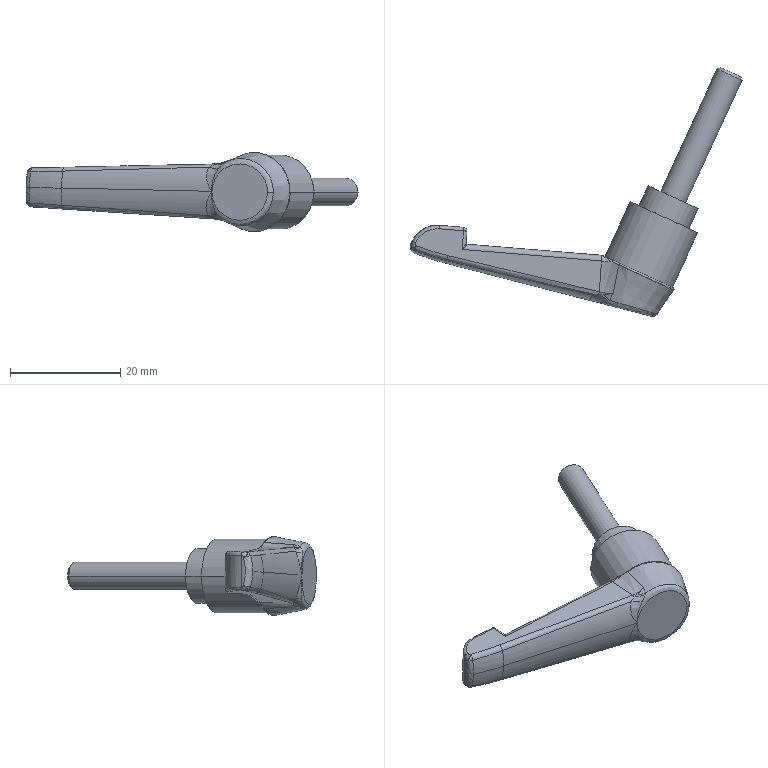Part | SolidWorks | features BaseBody 1 | 1 solid | 79 faces | box 60.381 x 45.237 x 14.385 mm | volume 5146 mm3 | spline 43 | cylinder 22 | plane 11 | cone 3 | commonest cylinder face diameters 1.2 x7 2 x3 10 x3 0.4 x2 5 x2 13.5 x2